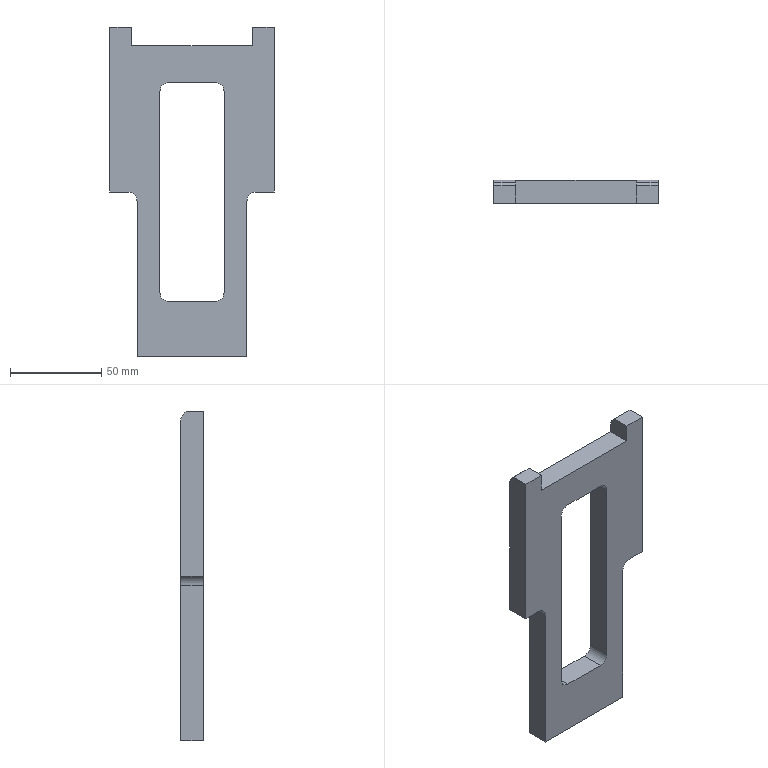Part | SolidWorks | features Fillet 3, Cut 2, Chamfer 1, Extrusion 1, ICE 1 | 1 solid | 28 faces | box 90 x 12.5 x 180 mm | volume 108281 mm3 | plane 20 | cylinder 8 | commonest cylinder face diameters 10 x8
STEP:
#1=CARTESIAN_POINT('',(45.,-6.25,180.));
#2=VERTEX_POINT('',#1);
#3=CARTESIAN_POINT('',(45.,3.25,180.));
#4=VERTEX_POINT('',#3);
#5=CARTESIAN_POINT('',(45.,6.25,180.));
#6=DIRECTION('',(0.,1.,0.));
#7=VECTOR('',#6,1000.);
#8=LINE('',#5,#7);
#9=EDGE_CURVE('',#2,#4,#8,.T.);
#10=ORIENTED_EDGE('',*,*,#9,.T.);
#11=CARTESIAN_POINT('',(33.,3.25,180.));
#12=VERTEX_POINT('',#11);
#13=CARTESIAN_POINT('',(33.,3.25,180.));
#14=DIRECTION('',(-1.,0.,0.));
#15=VECTOR('',#14,1000.);
#16=LINE('',#13,#15);
#17=EDGE_CURVE('',#4,#12,#16,.T.);
#18=ORIENTED_EDGE('',*,*,#17,.T.);
#19=CARTESIAN_POINT('',(33.,-6.25,180.));
#20=VERTEX_POINT('',#19);
#21=CARTESIAN_POINT('',(33.,-6.25,180.));
#22=DIRECTION('',(0.,1.,0.));
#23=VECTOR('',#22,1000.);
#24=LINE('',#21,#23);
#25=EDGE_CURVE('',#20,#12,#24,.T.);
#26=ORIENTED_EDGE('',*,*,#25,.F.);
#27=CARTESIAN_POINT('',(-45.,-6.25,180.));
#28=DIRECTION('',(1.,0.,0.));
#29=VECTOR('',#28,1000.);
#30=LINE('',#27,#29);
#31=EDGE_CURVE('',#20,#2,#30,.T.);
#32=ORIENTED_EDGE('',*,*,#31,.T.);
#33=EDGE_LOOP('',(#10,#18,#26,#32));
#34=FACE_OUTER_BOUND('',#33,.T.);
#35=CARTESIAN_POINT('',(0.,0.,180.));
#36=DIRECTION('',(0.,0.,1.));
#37=DIRECTION('',(1.,0.,0.));
#38=AXIS2_PLACEMENT_3D('',#35,#36,#37);
#39=PLANE('',#38);
#40=ADVANCED_FACE('',(#34),#39,.T.);
#41=CARTESIAN_POINT('',(-45.,6.25,174.929));
#42=VERTEX_POINT('',#41);
#43=CARTESIAN_POINT('',(-45.,6.25,90.));
#44=VERTEX_POINT('',#43);
#45=CARTESIAN_POINT('',(-45.,6.25,180.));
#46=DIRECTION('',(0.,0.,-1.));
#47=VECTOR('',#46,1000.);
#48=LINE('',#45,#47);
#49=EDGE_CURVE('',#42,#44,#48,.T.);
#50=ORIENTED_EDGE('',*,*,#49,.T.);
#51=CARTESIAN_POINT('',(-45.,-6.25,90.));
#52=VERTEX_POINT('',#51);
#53=CARTESIAN_POINT('',(-45.,-6.25,90.));
#54=DIRECTION('',(0.,1.,0.));
#55=VECTOR('',#54,1000.);
#56=LINE('',#53,#55);
#57=EDGE_CURVE('',#52,#44,#56,.T.);
#58=ORIENTED_EDGE('',*,*,#57,.F.);
#59=CARTESIAN_POINT('',(-45.,-6.25,180.));
#60=VERTEX_POINT('',#59);
#61=CARTESIAN_POINT('',(-45.,-6.25,180.));
#62=DIRECTION('',(0.,0.,-1.));
#63=VECTOR('',#62,1000.);
#64=LINE('',#61,#63);
#65=EDGE_CURVE('',#60,#52,#64,.T.);
#66=ORIENTED_EDGE('',*,*,#65,.F.);
#67=CARTESIAN_POINT('',(-45.,3.25,180.));
#68=VERTEX_POINT('',#67);
#69=CARTESIAN_POINT('',(-45.,6.25,180.));
#70=DIRECTION('',(0.,-1.,0.));
#71=VECTOR('',#70,1000.);
#72=LINE('',#69,#71);
#73=EDGE_CURVE('',#68,#60,#72,.T.);
#74=ORIENTED_EDGE('',*,*,#73,.F.);
#75=CARTESIAN_POINT('',(-45.,4.786,178.464));
#76=VERTEX_POINT('',#75);
#77=CARTESIAN_POINT('',(-45.,3.25,180.));
#78=DIRECTION('',(0.,0.7071,-0.7071));
#79=VECTOR('',#78,1000.);
#80=LINE('',#77,#79);
#81=EDGE_CURVE('',#68,#76,#80,.T.);
#82=ORIENTED_EDGE('',*,*,#81,.T.);
#83=CARTESIAN_POINT('',(-45.,1.25,174.929));
#84=DIRECTION('',(-1.,0.,0.));
#85=DIRECTION('',(0.,0.,-1.));
#86=AXIS2_PLACEMENT_3D('',#83,#84,#85);
#87=CIRCLE('',#86,5.);
#88=EDGE_CURVE('',#76,#42,#87,.T.);
#89=ORIENTED_EDGE('',*,*,#88,.T.);
#90=EDGE_LOOP('',(#50,#58,#66,#74,#82,#89));
#91=FACE_OUTER_BOUND('',#90,.T.);
#92=CARTESIAN_POINT('',(-45.,6.25,180.));
#93=DIRECTION('',(1.,0.,0.));
#94=DIRECTION('',(0.,0.,-1.));
#95=AXIS2_PLACEMENT_3D('',#92,#93,#94);
#96=PLANE('',#95);
#97=ADVANCED_FACE('',(#91),#96,.F.);
#98=CARTESIAN_POINT('',(17.5,-6.25,145.));
#99=VERTEX_POINT('',#98);
#100=CARTESIAN_POINT('',(17.5,-6.25,35.));
#101=VERTEX_POINT('',#100);
#102=CARTESIAN_POINT('',(17.5,-6.25,150.));
#103=DIRECTION('',(0.,0.,-1.));
#104=VECTOR('',#103,1000.);
#105=LINE('',#102,#104);
#106=EDGE_CURVE('',#99,#101,#105,.T.);
#107=ORIENTED_EDGE('',*,*,#106,.T.);
#108=CARTESIAN_POINT('',(12.5,-6.25,30.));
#109=VERTEX_POINT('',#108);
#110=CARTESIAN_POINT('',(12.5,-6.25,35.));
#111=DIRECTION('',(0.,1.,0.));
#112=DIRECTION('',(0.,0.,1.));
#113=AXIS2_PLACEMENT_3D('',#110,#111,#112);
#114=CIRCLE('',#113,5.);
#115=EDGE_CURVE('',#101,#109,#114,.T.);
#116=ORIENTED_EDGE('',*,*,#115,.T.);
#117=CARTESIAN_POINT('',(-12.5,-6.25,30.));
#118=VERTEX_POINT('',#117);
#119=CARTESIAN_POINT('',(-17.5,-6.25,30.));
#120=DIRECTION('',(-1.,0.,0.));
#121=VECTOR('',#120,1000.);
#122=LINE('',#119,#121);
#123=EDGE_CURVE('',#109,#118,#122,.T.);
#124=ORIENTED_EDGE('',*,*,#123,.T.);
#125=CARTESIAN_POINT('',(-17.5,-6.25,35.));
#126=VERTEX_POINT('',#125);
#127=CARTESIAN_POINT('',(-12.5,-6.25,35.));
#128=DIRECTION('',(0.,1.,0.));
#129=DIRECTION('',(0.,0.,1.));
#130=AXIS2_PLACEMENT_3D('',#127,#128,#129);
#131=CIRCLE('',#130,5.);
#132=EDGE_CURVE('',#118,#126,#131,.T.);
#133=ORIENTED_EDGE('',*,*,#132,.T.);
#134=CARTESIAN_POINT('',(-17.5,-6.25,145.));
#135=VERTEX_POINT('',#134);
#136=CARTESIAN_POINT('',(-17.5,-6.25,150.));
#137=DIRECTION('',(0.,0.,1.));
#138=VECTOR('',#137,1000.);
#139=LINE('',#136,#138);
#140=EDGE_CURVE('',#126,#135,#139,.T.);
#141=ORIENTED_EDGE('',*,*,#140,.T.);
#142=CARTESIAN_POINT('',(-12.5,-6.25,150.));
#143=VERTEX_POINT('',#142);
#144=CARTESIAN_POINT('',(-12.5,-6.25,145.));
#145=DIRECTION('',(0.,1.,0.));
#146=DIRECTION('',(0.,0.,1.));
#147=AXIS2_PLACEMENT_3D('',#144,#145,#146);
#148=CIRCLE('',#147,5.);
#149=EDGE_CURVE('',#135,#143,#148,.T.);
#150=ORIENTED_EDGE('',*,*,#149,.T.);
#151=CARTESIAN_POINT('',(12.5,-6.25,150.));
#152=VERTEX_POINT('',#151);
#153=CARTESIAN_POINT('',(-17.5,-6.25,150.));
#154=DIRECTION('',(1.,0.,0.));
#155=VECTOR('',#154,1000.);
#156=LINE('',#153,#155);
#157=EDGE_CURVE('',#143,#152,#156,.T.);
#158=ORIENTED_EDGE('',*,*,#157,.T.);
#159=CARTESIAN_POINT('',(12.5,-6.25,145.));
#160=DIRECTION('',(0.,1.,0.));
#161=DIRECTION('',(0.,0.,1.));
#162=AXIS2_PLACEMENT_3D('',#159,#160,#161);
#163=CIRCLE('',#162,5.);
#164=EDGE_CURVE('',#152,#99,#163,.T.);
#165=ORIENTED_EDGE('',*,*,#164,.T.);
#166=EDGE_LOOP('',(#107,#116,#124,#133,#141,#150,#158,#165));
#167=FACE_BOUND('',#166,.T.);
#168=CARTESIAN_POINT('',(-35.,-6.25,90.));
#169=VERTEX_POINT('',#168);
#170=CARTESIAN_POINT('',(-45.,-6.25,90.));
#171=DIRECTION('',(1.,0.,0.));
#172=VECTOR('',#171,1000.);
#173=LINE('',#170,#172);
#174=EDGE_CURVE('',#52,#169,#173,.T.);
#175=ORIENTED_EDGE('',*,*,#174,.T.);
#176=CARTESIAN_POINT('',(-30.,-6.25,85.));
#177=VERTEX_POINT('',#176);
#178=CARTESIAN_POINT('',(-35.,-6.25,85.));
#179=DIRECTION('',(0.,1.,0.));
#180=DIRECTION('',(0.,0.,1.));
#181=AXIS2_PLACEMENT_3D('',#178,#179,#180);
#182=CIRCLE('',#181,5.);
#183=EDGE_CURVE('',#169,#177,#182,.T.);
#184=ORIENTED_EDGE('',*,*,#183,.T.);
#185=CARTESIAN_POINT('',(-30.,-6.25,0.));
#186=VERTEX_POINT('',#185);
#187=CARTESIAN_POINT('',(-30.,-6.25,90.));
#188=DIRECTION('',(0.,0.,-1.));
#189=VECTOR('',#188,1000.);
#190=LINE('',#187,#189);
#191=EDGE_CURVE('',#177,#186,#190,.T.);
#192=ORIENTED_EDGE('',*,*,#191,.T.);
#193=CARTESIAN_POINT('',(30.,-6.25,0.));
#194=VERTEX_POINT('',#193);
#195=CARTESIAN_POINT('',(-45.,-6.25,0.));
#196=DIRECTION('',(1.,0.,0.));
#197=VECTOR('',#196,1000.);
#198=LINE('',#195,#197);
#199=EDGE_CURVE('',#186,#194,#198,.T.);
#200=ORIENTED_EDGE('',*,*,#199,.T.);
#201=CARTESIAN_POINT('',(30.,-6.25,85.));
#202=VERTEX_POINT('',#201);
#203=CARTESIAN_POINT('',(30.,-6.25,0.));
#204=DIRECTION('',(0.,0.,1.));
#205=VECTOR('',#204,1000.);
#206=LINE('',#203,#205);
#207=EDGE_CURVE('',#194,#202,#206,.T.);
#208=ORIENTED_EDGE('',*,*,#207,.T.);
#209=CARTESIAN_POINT('',(35.,-6.25,90.));
#210=VERTEX_POINT('',#209);
#211=CARTESIAN_POINT('',(35.,-6.25,85.));
#212=DIRECTION('',(0.,1.,0.));
#213=DIRECTION('',(0.,0.,1.));
#214=AXIS2_PLACEMENT_3D('',#211,#212,#213);
#215=CIRCLE('',#214,5.);
#216=EDGE_CURVE('',#202,#210,#215,.T.);
#217=ORIENTED_EDGE('',*,*,#216,.T.);
#218=CARTESIAN_POINT('',(45.,-6.25,90.));
#219=VERTEX_POINT('',#218);
#220=CARTESIAN_POINT('',(45.,-6.25,90.));
#221=DIRECTION('',(1.,0.,0.));
#222=VECTOR('',#221,1000.);
#223=LINE('',#220,#222);
#224=EDGE_CURVE('',#210,#219,#223,.T.);
#225=ORIENTED_EDGE('',*,*,#224,.T.);
#226=CARTESIAN_POINT('',(45.,-6.25,180.));
#227=DIRECTION('',(0.,0.,-1.));
#228=VECTOR('',#227,1000.);
#229=LINE('',#226,#228);
#230=EDGE_CURVE('',#2,#219,#229,.T.);
#231=ORIENTED_EDGE('',*,*,#230,.F.);
#232=ORIENTED_EDGE('',*,*,#31,.F.);
#233=CARTESIAN_POINT('',(33.,-6.25,170.));
#234=VERTEX_POINT('',#233);
#235=CARTESIAN_POINT('',(33.,-6.25,180.));
#236=DIRECTION('',(0.,0.,-1.));
#237=VECTOR('',#236,1000.);
#238=LINE('',#235,#237);
#239=EDGE_CURVE('',#20,#234,#238,.T.);
#240=ORIENTED_EDGE('',*,*,#239,.T.);
#241=CARTESIAN_POINT('',(-33.,-6.25,170.));
#242=VERTEX_POINT('',#241);
#243=CARTESIAN_POINT('',(33.,-6.25,170.));
#244=DIRECTION('',(-1.,0.,0.));
#245=VECTOR('',#244,1000.);
#246=LINE('',#243,#245);
#247=EDGE_CURVE('',#234,#242,#246,.T.);
#248=ORIENTED_EDGE('',*,*,#247,.T.);
#249=CARTESIAN_POINT('',(-33.,-6.25,180.));
#250=VERTEX_POINT('',#249);
#251=CARTESIAN_POINT('',(-33.,-6.25,180.));
#252=DIRECTION('',(0.,0.,1.));
#253=VECTOR('',#252,1000.);
#254=LINE('',#251,#253);
#255=EDGE_CURVE('',#242,#250,#254,.T.);
#256=ORIENTED_EDGE('',*,*,#255,.T.);
#257=CARTESIAN_POINT('',(-45.,-6.25,180.));
#258=DIRECTION('',(1.,0.,0.));
#259=VECTOR('',#258,1000.);
#260=LINE('',#257,#259);
#261=EDGE_CURVE('',#60,#250,#260,.T.);
#262=ORIENTED_EDGE('',*,*,#261,.F.);
#263=ORIENTED_EDGE('',*,*,#65,.T.);
#264=EDGE_LOOP('',(#175,#184,#192,#200,#208,#217,#225,#231,#232,#240,#248,#256,#262,#263));
#265=FACE_OUTER_BOUND('',#264,.T.);
#266=CARTESIAN_POINT('',(-45.,-6.25,180.));
#267=DIRECTION('',(0.,1.,0.));
#268=DIRECTION('',(0.,0.,1.));
#269=AXIS2_PLACEMENT_3D('',#266,#267,#268);
#270=PLANE('',#269);
#271=ADVANCED_FACE('',(#167,#265),#270,.F.);
#272=ORIENTED_EDGE('',*,*,#230,.T.);
#273=CARTESIAN_POINT('',(45.,6.25,90.));
#274=VERTEX_POINT('',#273);
#275=CARTESIAN_POINT('',(45.,-6.25,90.));
#276=DIRECTION('',(0.,1.,0.));
#277=VECTOR('',#276,1000.);
#278=LINE('',#275,#277);
#279=EDGE_CURVE('',#219,#274,#278,.T.);
#280=ORIENTED_EDGE('',*,*,#279,.T.);
#281=CARTESIAN_POINT('',(45.,6.25,174.929));
#282=VERTEX_POINT('',#281);
#283=CARTESIAN_POINT('',(45.,6.25,180.));
#284=DIRECTION('',(0.,0.,-1.));
#285=VECTOR('',#284,1000.);
#286=LINE('',#283,#285);
#287=EDGE_CURVE('',#282,#274,#286,.T.);
#288=ORIENTED_EDGE('',*,*,#287,.F.);
#289=CARTESIAN_POINT('',(45.,4.786,178.464));
#290=VERTEX_POINT('',#289);
#291=CARTESIAN_POINT('',(45.,1.25,174.929));
#292=DIRECTION('',(1.,0.,0.));
#293=DIRECTION('',(0.,0.,1.));
#294=AXIS2_PLACEMENT_3D('',#291,#292,#293);
#295=CIRCLE('',#294,5.);
#296=EDGE_CURVE('',#282,#290,#295,.T.);
#297=ORIENTED_EDGE('',*,*,#296,.T.);
#298=CARTESIAN_POINT('',(45.,3.25,180.));
#299=DIRECTION('',(0.,-0.7071,0.7071));
#300=VECTOR('',#299,1000.);
#301=LINE('',#298,#300);
#302=EDGE_CURVE('',#290,#4,#301,.T.);
#303=ORIENTED_EDGE('',*,*,#302,.T.);
#304=ORIENTED_EDGE('',*,*,#9,.F.);
#305=EDGE_LOOP('',(#272,#280,#288,#297,#303,#304));
#306=FACE_OUTER_BOUND('',#305,.T.);
#307=CARTESIAN_POINT('',(45.,6.25,180.));
#308=DIRECTION('',(-1.,0.,0.));
#309=DIRECTION('',(0.,0.,1.));
#310=AXIS2_PLACEMENT_3D('',#307,#308,#309);
#311=PLANE('',#310);
#312=ADVANCED_FACE('',(#306),#311,.F.);
#313=CARTESIAN_POINT('',(-12.5,6.25,150.));
#314=VERTEX_POINT('',#313);
#315=CARTESIAN_POINT('',(12.5,6.25,150.));
#316=VERTEX_POINT('',#315);
#317=CARTESIAN_POINT('',(-17.5,6.25,150.));
#318=DIRECTION('',(1.,0.,0.));
#319=VECTOR('',#318,1000.);
#320=LINE('',#317,#319);
#321=EDGE_CURVE('',#314,#316,#320,.T.);
#322=ORIENTED_EDGE('',*,*,#321,.F.);
#323=CARTESIAN_POINT('',(-17.5,6.25,145.));
#324=VERTEX_POINT('',#323);
#325=CARTESIAN_POINT('',(-12.5,6.25,145.));
#326=DIRECTION('',(0.,-1.,0.));
#327=DIRECTION('',(1.,0.,0.));
#328=AXIS2_PLACEMENT_3D('',#325,#326,#327);
#329=CIRCLE('',#328,5.);
#330=EDGE_CURVE('',#314,#324,#329,.T.);
#331=ORIENTED_EDGE('',*,*,#330,.T.);
#332=CARTESIAN_POINT('',(-17.5,6.25,35.));
#333=VERTEX_POINT('',#332);
#334=CARTESIAN_POINT('',(-17.5,6.25,150.));
#335=DIRECTION('',(0.,0.,1.));
#336=VECTOR('',#335,1000.);
#337=LINE('',#334,#336);
#338=EDGE_CURVE('',#333,#324,#337,.T.);
#339=ORIENTED_EDGE('',*,*,#338,.F.);
#340=CARTESIAN_POINT('',(-12.5,6.25,30.));
#341=VERTEX_POINT('',#340);
#342=CARTESIAN_POINT('',(-12.5,6.25,35.));
#343=DIRECTION('',(0.,-1.,0.));
#344=DIRECTION('',(1.,0.,0.));
#345=AXIS2_PLACEMENT_3D('',#342,#343,#344);
#346=CIRCLE('',#345,5.);
#347=EDGE_CURVE('',#333,#341,#346,.T.);
#348=ORIENTED_EDGE('',*,*,#347,.T.);
#349=CARTESIAN_POINT('',(12.5,6.25,30.));
#350=VERTEX_POINT('',#349);
#351=CARTESIAN_POINT('',(-17.5,6.25,30.));
#352=DIRECTION('',(-1.,0.,0.));
#353=VECTOR('',#352,1000.);
#354=LINE('',#351,#353);
#355=EDGE_CURVE('',#350,#341,#354,.T.);
#356=ORIENTED_EDGE('',*,*,#355,.F.);
#357=CARTESIAN_POINT('',(17.5,6.25,35.));
#358=VERTEX_POINT('',#357);
#359=CARTESIAN_POINT('',(12.5,6.25,35.));
#360=DIRECTION('',(0.,-1.,0.));
#361=DIRECTION('',(1.,0.,0.));
#362=AXIS2_PLACEMENT_3D('',#359,#360,#361);
#363=CIRCLE('',#362,5.);
#364=EDGE_CURVE('',#350,#358,#363,.T.);
#365=ORIENTED_EDGE('',*,*,#364,.T.);
#366=CARTESIAN_POINT('',(17.5,6.25,145.));
#367=VERTEX_POINT('',#366);
#368=CARTESIAN_POINT('',(17.5,6.25,150.));
#369=DIRECTION('',(0.,0.,-1.));
#370=VECTOR('',#369,1000.);
#371=LINE('',#368,#370);
#372=EDGE_CURVE('',#367,#358,#371,.T.);
#373=ORIENTED_EDGE('',*,*,#372,.F.);
#374=CARTESIAN_POINT('',(12.5,6.25,145.));
#375=DIRECTION('',(0.,-1.,0.));
#376=DIRECTION('',(1.,0.,0.));
#377=AXIS2_PLACEMENT_3D('',#374,#375,#376);
#378=CIRCLE('',#377,5.);
#379=EDGE_CURVE('',#367,#316,#378,.T.);
#380=ORIENTED_EDGE('',*,*,#379,.T.);
#381=EDGE_LOOP('',(#322,#331,#339,#348,#356,#365,#373,#380));
#382=FACE_BOUND('',#381,.T.);
#383=CARTESIAN_POINT('',(30.,6.25,0.));
#384=VERTEX_POINT('',#383);
#385=CARTESIAN_POINT('',(-30.,6.25,0.));
#386=VERTEX_POINT('',#385);
#387=CARTESIAN_POINT('',(-45.,6.25,0.));
#388=DIRECTION('',(-1.,0.,0.));
#389=VECTOR('',#388,1000.);
#390=LINE('',#387,#389);
#391=EDGE_CURVE('',#384,#386,#390,.T.);
#392=ORIENTED_EDGE('',*,*,#391,.T.);
#393=CARTESIAN_POINT('',(-30.,6.25,85.));
#394=VERTEX_POINT('',#393);
#395=CARTESIAN_POINT('',(-30.,6.25,90.));
#396=DIRECTION('',(0.,0.,-1.));
#397=VECTOR('',#396,1000.);
#398=LINE('',#395,#397);
#399=EDGE_CURVE('',#394,#386,#398,.T.);
#400=ORIENTED_EDGE('',*,*,#399,.F.);
#401=CARTESIAN_POINT('',(-35.,6.25,90.));
#402=VERTEX_POINT('',#401);
#403=CARTESIAN_POINT('',(-35.,6.25,85.));
#404=DIRECTION('',(0.,-1.,0.));
#405=DIRECTION('',(1.,0.,0.));
#406=AXIS2_PLACEMENT_3D('',#403,#404,#405);
#407=CIRCLE('',#406,5.);
#408=EDGE_CURVE('',#394,#402,#407,.T.);
#409=ORIENTED_EDGE('',*,*,#408,.T.);
#410=CARTESIAN_POINT('',(-45.,6.25,90.));
#411=DIRECTION('',(1.,0.,0.));
#412=VECTOR('',#411,1000.);
#413=LINE('',#410,#412);
#414=EDGE_CURVE('',#44,#402,#413,.T.);
#415=ORIENTED_EDGE('',*,*,#414,.F.);
#416=ORIENTED_EDGE('',*,*,#49,.F.);
#417=CARTESIAN_POINT('',(-33.,6.25,174.929));
#418=VERTEX_POINT('',#417);
#419=CARTESIAN_POINT('',(-33.,6.25,174.929));
#420=DIRECTION('',(1.,0.,0.));
#421=VECTOR('',#420,1000.);
#422=LINE('',#419,#421);
#423=EDGE_CURVE('',#42,#418,#422,.T.);
#424=ORIENTED_EDGE('',*,*,#423,.T.);
#425=CARTESIAN_POINT('',(-33.,6.25,170.));
#426=VERTEX_POINT('',#425);
#427=CARTESIAN_POINT('',(-33.,6.25,180.));
#428=DIRECTION('',(0.,0.,1.));
#429=VECTOR('',#428,1000.);
#430=LINE('',#427,#429);
#431=EDGE_CURVE('',#426,#418,#430,.T.);
#432=ORIENTED_EDGE('',*,*,#431,.F.);
#433=CARTESIAN_POINT('',(33.,6.25,170.));
#434=VERTEX_POINT('',#433);
#435=CARTESIAN_POINT('',(33.,6.25,170.));
#436=DIRECTION('',(-1.,0.,0.));
#437=VECTOR('',#436,1000.);
#438=LINE('',#435,#437);
#439=EDGE_CURVE('',#434,#426,#438,.T.);
#440=ORIENTED_EDGE('',*,*,#439,.F.);
#441=CARTESIAN_POINT('',(33.,6.25,174.929));
#442=VERTEX_POINT('',#441);
#443=CARTESIAN_POINT('',(33.,6.25,180.));
#444=DIRECTION('',(0.,0.,-1.));
#445=VECTOR('',#444,1000.);
#446=LINE('',#443,#445);
#447=EDGE_CURVE('',#442,#434,#446,.T.);
#448=ORIENTED_EDGE('',*,*,#447,.F.);
#449=CARTESIAN_POINT('',(45.,6.25,174.929));
#450=DIRECTION('',(1.,0.,0.));
#451=VECTOR('',#450,1000.);
#452=LINE('',#449,#451);
#453=EDGE_CURVE('',#442,#282,#452,.T.);
#454=ORIENTED_EDGE('',*,*,#453,.T.);
#455=ORIENTED_EDGE('',*,*,#287,.T.);
#456=CARTESIAN_POINT('',(35.,6.25,90.));
#457=VERTEX_POINT('',#456);
#458=CARTESIAN_POINT('',(45.,6.25,90.));
#459=DIRECTION('',(1.,0.,0.));
#460=VECTOR('',#459,1000.);
#461=LINE('',#458,#460);
#462=EDGE_CURVE('',#457,#274,#461,.T.);
#463=ORIENTED_EDGE('',*,*,#462,.F.);
#464=CARTESIAN_POINT('',(30.,6.25,85.));
#465=VERTEX_POINT('',#464);
#466=CARTESIAN_POINT('',(35.,6.25,85.));
#467=DIRECTION('',(0.,-1.,0.));
#468=DIRECTION('',(1.,0.,0.));
#469=AXIS2_PLACEMENT_3D('',#466,#467,#468);
#470=CIRCLE('',#469,5.);
#471=EDGE_CURVE('',#457,#465,#470,.T.);
#472=ORIENTED_EDGE('',*,*,#471,.T.);
#473=CARTESIAN_POINT('',(30.,6.25,0.));
#474=DIRECTION('',(0.,0.,1.));
#475=VECTOR('',#474,1000.);
#476=LINE('',#473,#475);
#477=EDGE_CURVE('',#384,#465,#476,.T.);
#478=ORIENTED_EDGE('',*,*,#477,.F.);
#479=EDGE_LOOP('',(#392,#400,#409,#415,#416,#424,#432,#440,#448,#454,#455,#463,#472,#478));
#480=FACE_OUTER_BOUND('',#479,.T.);
#481=CARTESIAN_POINT('',(-45.,6.25,180.));
#482=DIRECTION('',(0.,-1.,0.));
#483=DIRECTION('',(1.,0.,0.));
#484=AXIS2_PLACEMENT_3D('',#481,#482,#483);
#485=PLANE('',#484);
#486=ADVANCED_FACE('',(#382,#480),#485,.F.);
#487=CARTESIAN_POINT('',(-33.,3.25,180.));
#488=VERTEX_POINT('',#487);
#489=CARTESIAN_POINT('',(-33.,-6.25,180.));
#490=DIRECTION('',(0.,1.,0.));
#491=VECTOR('',#490,1000.);
#492=LINE('',#489,#491);
#493=EDGE_CURVE('',#250,#488,#492,.T.);
#494=ORIENTED_EDGE('',*,*,#493,.T.);
#495=CARTESIAN_POINT('',(-45.,3.25,180.));
#496=DIRECTION('',(-1.,0.,0.));
#497=VECTOR('',#496,1000.);
#498=LINE('',#495,#497);
#499=EDGE_CURVE('',#488,#68,#498,.T.);
#500=ORIENTED_EDGE('',*,*,#499,.T.);
#501=ORIENTED_EDGE('',*,*,#73,.T.);
#502=ORIENTED_EDGE('',*,*,#261,.T.);
#503=EDGE_LOOP('',(#494,#500,#501,#502));
#504=FACE_OUTER_BOUND('',#503,.T.);
#505=CARTESIAN_POINT('',(0.,0.,180.));
#506=DIRECTION('',(0.,0.,1.));
#507=DIRECTION('',(1.,0.,0.));
#508=AXIS2_PLACEMENT_3D('',#505,#506,#507);
#509=PLANE('',#508);
#510=ADVANCED_FACE('',(#504),#509,.T.);
#511=ORIENTED_EDGE('',*,*,#199,.F.);
#512=CARTESIAN_POINT('',(-30.,-6.25,0.));
#513=DIRECTION('',(0.,1.,0.));
#514=VECTOR('',#513,1000.);
#515=LINE('',#512,#514);
#516=EDGE_CURVE('',#186,#386,#515,.T.);
#517=ORIENTED_EDGE('',*,*,#516,.T.);
#518=ORIENTED_EDGE('',*,*,#391,.F.);
#519=CARTESIAN_POINT('',(30.,-6.25,0.));
#520=DIRECTION('',(0.,1.,0.));
#521=VECTOR('',#520,1000.);
#522=LINE('',#519,#521);
#523=EDGE_CURVE('',#194,#384,#522,.T.);
#524=ORIENTED_EDGE('',*,*,#523,.F.);
#525=EDGE_LOOP('',(#511,#517,#518,#524));
#526=FACE_OUTER_BOUND('',#525,.T.);
#527=CARTESIAN_POINT('',(0.,0.,0.));
#528=DIRECTION('',(0.,0.,1.));
#529=DIRECTION('',(1.,0.,0.));
#530=AXIS2_PLACEMENT_3D('',#527,#528,#529);
#531=PLANE('',#530);
#532=ADVANCED_FACE('',(#526),#531,.F.);
#533=CARTESIAN_POINT('',(33.,4.786,178.464));
#534=VERTEX_POINT('',#533);
#535=CARTESIAN_POINT('',(33.,3.25,180.));
#536=DIRECTION('',(0.,0.7071,-0.7071));
#537=VECTOR('',#536,1000.);
#538=LINE('',#535,#537);
#539=EDGE_CURVE('',#12,#534,#538,.T.);
#540=ORIENTED_EDGE('',*,*,#539,.T.);
#541=CARTESIAN_POINT('',(33.,1.25,174.929));
#542=DIRECTION('',(-1.,0.,0.));
#543=DIRECTION('',(0.,1.,0.));
#544=AXIS2_PLACEMENT_3D('',#541,#542,#543);
#545=CIRCLE('',#544,5.);
#546=EDGE_CURVE('',#534,#442,#545,.T.);
#547=ORIENTED_EDGE('',*,*,#546,.T.);
#548=ORIENTED_EDGE('',*,*,#447,.T.);
#549=CARTESIAN_POINT('',(33.,-6.25,170.));
#550=DIRECTION('',(0.,1.,0.));
#551=VECTOR('',#550,1000.);
#552=LINE('',#549,#551);
#553=EDGE_CURVE('',#234,#434,#552,.T.);
#554=ORIENTED_EDGE('',*,*,#553,.F.);
#555=ORIENTED_EDGE('',*,*,#239,.F.);
#556=ORIENTED_EDGE('',*,*,#25,.T.);
#557=EDGE_LOOP('',(#540,#547,#548,#554,#555,#556));
#558=FACE_OUTER_BOUND('',#557,.T.);
#559=CARTESIAN_POINT('',(33.,-6.25,180.));
#560=DIRECTION('',(1.,0.,0.));
#561=DIRECTION('',(0.,1.,0.));
#562=AXIS2_PLACEMENT_3D('',#559,#560,#561);
#563=PLANE('',#562);
#564=ADVANCED_FACE('',(#558),#563,.F.);
#565=ORIENTED_EDGE('',*,*,#431,.T.);
#566=CARTESIAN_POINT('',(-33.,4.786,178.464));
#567=VERTEX_POINT('',#566);
#568=CARTESIAN_POINT('',(-33.,1.25,174.929));
#569=DIRECTION('',(1.,0.,0.));
#570=DIRECTION('',(0.,-1.,0.));
#571=AXIS2_PLACEMENT_3D('',#568,#569,#570);
#572=CIRCLE('',#571,5.);
#573=EDGE_CURVE('',#418,#567,#572,.T.);
#574=ORIENTED_EDGE('',*,*,#573,.T.);
#575=CARTESIAN_POINT('',(-33.,3.25,180.));
#576=DIRECTION('',(0.,-0.7071,0.7071));
#577=VECTOR('',#576,1000.);
#578=LINE('',#575,#577);
#579=EDGE_CURVE('',#567,#488,#578,.T.);
#580=ORIENTED_EDGE('',*,*,#579,.T.);
#581=ORIENTED_EDGE('',*,*,#493,.F.);
#582=ORIENTED_EDGE('',*,*,#255,.F.);
#583=CARTESIAN_POINT('',(-33.,-6.25,170.));
#584=DIRECTION('',(0.,1.,0.));
#585=VECTOR('',#584,1000.);
#586=LINE('',#583,#585);
#587=EDGE_CURVE('',#242,#426,#586,.T.);
#588=ORIENTED_EDGE('',*,*,#587,.T.);
#589=EDGE_LOOP('',(#565,#574,#580,#581,#582,#588));
#590=FACE_OUTER_BOUND('',#589,.T.);
#591=CARTESIAN_POINT('',(-33.,-6.25,180.));
#592=DIRECTION('',(-1.,0.,0.));
#593=DIRECTION('',(0.,-1.,0.));
#594=AXIS2_PLACEMENT_3D('',#591,#592,#593);
#595=PLANE('',#594);
#596=ADVANCED_FACE('',(#590),#595,.F.);
#597=ORIENTED_EDGE('',*,*,#439,.T.);
#598=ORIENTED_EDGE('',*,*,#587,.F.);
#599=ORIENTED_EDGE('',*,*,#247,.F.);
#600=ORIENTED_EDGE('',*,*,#553,.T.);
#601=EDGE_LOOP('',(#597,#598,#599,#600));
#602=FACE_OUTER_BOUND('',#601,.T.);
#603=CARTESIAN_POINT('',(33.,-6.25,170.));
#604=DIRECTION('',(0.,0.,-1.));
#605=DIRECTION('',(-1.,0.,0.));
#606=AXIS2_PLACEMENT_3D('',#603,#604,#605);
#607=PLANE('',#606);
#608=ADVANCED_FACE('',(#602),#607,.F.);
#609=ORIENTED_EDGE('',*,*,#579,.F.);
#610=CARTESIAN_POINT('',(-45.,4.786,178.464));
#611=DIRECTION('',(-1.,0.,0.));
#612=VECTOR('',#611,1000.);
#613=LINE('',#610,#612);
#614=EDGE_CURVE('',#567,#76,#613,.T.);
#615=ORIENTED_EDGE('',*,*,#614,.T.);
#616=ORIENTED_EDGE('',*,*,#81,.F.);
#617=ORIENTED_EDGE('',*,*,#499,.F.);
#618=EDGE_LOOP('',(#609,#615,#616,#617));
#619=FACE_OUTER_BOUND('',#618,.T.);
#620=CARTESIAN_POINT('',(0.,3.25,180.));
#621=DIRECTION('',(0.,0.7071,0.7071));
#622=DIRECTION('',(1.,0.,0.));
#623=AXIS2_PLACEMENT_3D('',#620,#621,#622);
#624=PLANE('',#623);
#625=ADVANCED_FACE('',(#619),#624,.T.);
#626=ORIENTED_EDGE('',*,*,#302,.F.);
#627=CARTESIAN_POINT('',(33.,4.786,178.464));
#628=DIRECTION('',(-1.,0.,0.));
#629=VECTOR('',#628,1000.);
#630=LINE('',#627,#629);
#631=EDGE_CURVE('',#290,#534,#630,.T.);
#632=ORIENTED_EDGE('',*,*,#631,.T.);
#633=ORIENTED_EDGE('',*,*,#539,.F.);
#634=ORIENTED_EDGE('',*,*,#17,.F.);
#635=EDGE_LOOP('',(#626,#632,#633,#634));
#636=FACE_OUTER_BOUND('',#635,.T.);
#637=CARTESIAN_POINT('',(0.,3.25,180.));
#638=DIRECTION('',(0.,0.7071,0.7071));
#639=DIRECTION('',(1.,0.,0.));
#640=AXIS2_PLACEMENT_3D('',#637,#638,#639);
#641=PLANE('',#640);
#642=ADVANCED_FACE('',(#636),#641,.T.);
#643=ORIENTED_EDGE('',*,*,#88,.F.);
#644=ORIENTED_EDGE('',*,*,#614,.F.);
#645=ORIENTED_EDGE('',*,*,#573,.F.);
#646=ORIENTED_EDGE('',*,*,#423,.F.);
#647=EDGE_LOOP('',(#643,#644,#645,#646));
#648=FACE_OUTER_BOUND('',#647,.T.);
#649=CARTESIAN_POINT('',(-45.,1.25,174.929));
#650=DIRECTION('',(-1.,0.,0.));
#651=DIRECTION('',(0.,-1.,0.));
#652=AXIS2_PLACEMENT_3D('',#649,#650,#651);
#653=CYLINDRICAL_SURFACE('',#652,5.);
#654=ADVANCED_FACE('',(#648),#653,.T.);
#655=ORIENTED_EDGE('',*,*,#546,.F.);
#656=ORIENTED_EDGE('',*,*,#631,.F.);
#657=ORIENTED_EDGE('',*,*,#296,.F.);
#658=ORIENTED_EDGE('',*,*,#453,.F.);
#659=EDGE_LOOP('',(#655,#656,#657,#658));
#660=FACE_OUTER_BOUND('',#659,.T.);
#661=CARTESIAN_POINT('',(-45.,1.25,174.929));
#662=DIRECTION('',(-1.,0.,0.));
#663=DIRECTION('',(0.,-1.,0.));
#664=AXIS2_PLACEMENT_3D('',#661,#662,#663);
#665=CYLINDRICAL_SURFACE('',#664,5.);
#666=ADVANCED_FACE('',(#660),#665,.T.);
#667=ORIENTED_EDGE('',*,*,#224,.F.);
#668=CARTESIAN_POINT('',(35.,6.25,90.));
#669=DIRECTION('',(0.,1.,0.));
#670=VECTOR('',#669,1000.);
#671=LINE('',#668,#670);
#672=EDGE_CURVE('',#210,#457,#671,.T.);
#673=ORIENTED_EDGE('',*,*,#672,.T.);
#674=ORIENTED_EDGE('',*,*,#462,.T.);
#675=ORIENTED_EDGE('',*,*,#279,.F.);
#676=EDGE_LOOP('',(#667,#673,#674,#675));
#677=FACE_OUTER_BOUND('',#676,.T.);
#678=CARTESIAN_POINT('',(45.,-6.25,90.));
#679=DIRECTION('',(0.,0.,1.));
#680=DIRECTION('',(1.,0.,0.));
#681=AXIS2_PLACEMENT_3D('',#678,#679,#680);
#682=PLANE('',#681);
#683=ADVANCED_FACE('',(#677),#682,.F.);
#684=ORIENTED_EDGE('',*,*,#477,.T.);
#685=CARTESIAN_POINT('',(30.,-6.25,85.));
#686=DIRECTION('',(0.,-1.,0.));
#687=VECTOR('',#686,1000.);
#688=LINE('',#685,#687);
#689=EDGE_CURVE('',#465,#202,#688,.T.);
#690=ORIENTED_EDGE('',*,*,#689,.T.);
#691=ORIENTED_EDGE('',*,*,#207,.F.);
#692=ORIENTED_EDGE('',*,*,#523,.T.);
#693=EDGE_LOOP('',(#684,#690,#691,#692));
#694=FACE_OUTER_BOUND('',#693,.T.);
#695=CARTESIAN_POINT('',(30.,-6.25,0.));
#696=DIRECTION('',(-1.,0.,0.));
#697=DIRECTION('',(0.,-1.,0.));
#698=AXIS2_PLACEMENT_3D('',#695,#696,#697);
#699=PLANE('',#698);
#700=ADVANCED_FACE('',(#694),#699,.F.);
#701=ORIENTED_EDGE('',*,*,#191,.F.);
#702=CARTESIAN_POINT('',(-30.,6.25,85.));
#703=DIRECTION('',(0.,1.,0.));
#704=VECTOR('',#703,1000.);
#705=LINE('',#702,#704);
#706=EDGE_CURVE('',#177,#394,#705,.T.);
#707=ORIENTED_EDGE('',*,*,#706,.T.);
#708=ORIENTED_EDGE('',*,*,#399,.T.);
#709=ORIENTED_EDGE('',*,*,#516,.F.);
#710=EDGE_LOOP('',(#701,#707,#708,#709));
#711=FACE_OUTER_BOUND('',#710,.T.);
#712=CARTESIAN_POINT('',(-30.,-6.25,90.));
#713=DIRECTION('',(1.,0.,0.));
#714=DIRECTION('',(0.,1.,0.));
#715=AXIS2_PLACEMENT_3D('',#712,#713,#714);
#716=PLANE('',#715);
#717=ADVANCED_FACE('',(#711),#716,.F.);
#718=ORIENTED_EDGE('',*,*,#414,.T.);
#719=CARTESIAN_POINT('',(-35.,-6.25,90.));
#720=DIRECTION('',(0.,-1.,0.));
#721=VECTOR('',#720,1000.);
#722=LINE('',#719,#721);
#723=EDGE_CURVE('',#402,#169,#722,.T.);
#724=ORIENTED_EDGE('',*,*,#723,.T.);
#725=ORIENTED_EDGE('',*,*,#174,.F.);
#726=ORIENTED_EDGE('',*,*,#57,.T.);
#727=EDGE_LOOP('',(#718,#724,#725,#726));
#728=FACE_OUTER_BOUND('',#727,.T.);
#729=CARTESIAN_POINT('',(-45.,-6.25,90.));
#730=DIRECTION('',(0.,0.,1.));
#731=DIRECTION('',(1.,0.,0.));
#732=AXIS2_PLACEMENT_3D('',#729,#730,#731);
#733=PLANE('',#732);
#734=ADVANCED_FACE('',(#728),#733,.F.);
#735=ORIENTED_EDGE('',*,*,#140,.F.);
#736=CARTESIAN_POINT('',(-17.5,6.25,35.));
#737=DIRECTION('',(0.,1.,0.));
#738=VECTOR('',#737,1000.);
#739=LINE('',#736,#738);
#740=EDGE_CURVE('',#126,#333,#739,.T.);
#741=ORIENTED_EDGE('',*,*,#740,.T.);
#742=ORIENTED_EDGE('',*,*,#338,.T.);
#743=CARTESIAN_POINT('',(-17.5,-6.25,145.));
#744=DIRECTION('',(0.,-1.,0.));
#745=VECTOR('',#744,1000.);
#746=LINE('',#743,#745);
#747=EDGE_CURVE('',#324,#135,#746,.T.);
#748=ORIENTED_EDGE('',*,*,#747,.T.);
#749=EDGE_LOOP('',(#735,#741,#742,#748));
#750=FACE_OUTER_BOUND('',#749,.T.);
#751=CARTESIAN_POINT('',(-17.5,-6.25,150.));
#752=DIRECTION('',(-1.,0.,0.));
#753=DIRECTION('',(0.,-1.,0.));
#754=AXIS2_PLACEMENT_3D('',#751,#752,#753);
#755=PLANE('',#754);
#756=ADVANCED_FACE('',(#750),#755,.F.);
#757=ORIENTED_EDGE('',*,*,#123,.F.);
#758=CARTESIAN_POINT('',(12.5,6.25,30.));
#759=DIRECTION('',(0.,1.,0.));
#760=VECTOR('',#759,1000.);
#761=LINE('',#758,#760);
#762=EDGE_CURVE('',#109,#350,#761,.T.);
#763=ORIENTED_EDGE('',*,*,#762,.T.);
#764=ORIENTED_EDGE('',*,*,#355,.T.);
#765=CARTESIAN_POINT('',(-12.5,-6.25,30.));
#766=DIRECTION('',(0.,-1.,0.));
#767=VECTOR('',#766,1000.);
#768=LINE('',#765,#767);
#769=EDGE_CURVE('',#341,#118,#768,.T.);
#770=ORIENTED_EDGE('',*,*,#769,.T.);
#771=EDGE_LOOP('',(#757,#763,#764,#770));
#772=FACE_OUTER_BOUND('',#771,.T.);
#773=CARTESIAN_POINT('',(-17.5,-6.25,30.));
#774=DIRECTION('',(0.,0.,-1.));
#775=DIRECTION('',(-1.,0.,0.));
#776=AXIS2_PLACEMENT_3D('',#773,#774,#775);
#777=PLANE('',#776);
#778=ADVANCED_FACE('',(#772),#777,.F.);
#779=ORIENTED_EDGE('',*,*,#372,.T.);
#780=CARTESIAN_POINT('',(17.5,-6.25,35.));
#781=DIRECTION('',(0.,-1.,0.));
#782=VECTOR('',#781,1000.);
#783=LINE('',#780,#782);
#784=EDGE_CURVE('',#358,#101,#783,.T.);
#785=ORIENTED_EDGE('',*,*,#784,.T.);
#786=ORIENTED_EDGE('',*,*,#106,.F.);
#787=CARTESIAN_POINT('',(17.5,6.25,145.));
#788=DIRECTION('',(0.,1.,0.));
#789=VECTOR('',#788,1000.);
#790=LINE('',#787,#789);
#791=EDGE_CURVE('',#99,#367,#790,.T.);
#792=ORIENTED_EDGE('',*,*,#791,.T.);
#793=EDGE_LOOP('',(#779,#785,#786,#792));
#794=FACE_OUTER_BOUND('',#793,.T.);
#795=CARTESIAN_POINT('',(17.5,-6.25,150.));
#796=DIRECTION('',(1.,0.,0.));
#797=DIRECTION('',(0.,1.,0.));
#798=AXIS2_PLACEMENT_3D('',#795,#796,#797);
#799=PLANE('',#798);
#800=ADVANCED_FACE('',(#794),#799,.F.);
#801=ORIENTED_EDGE('',*,*,#321,.T.);
#802=CARTESIAN_POINT('',(12.5,-6.25,150.));
#803=DIRECTION('',(0.,-1.,0.));
#804=VECTOR('',#803,1000.);
#805=LINE('',#802,#804);
#806=EDGE_CURVE('',#316,#152,#805,.T.);
#807=ORIENTED_EDGE('',*,*,#806,.T.);
#808=ORIENTED_EDGE('',*,*,#157,.F.);
#809=CARTESIAN_POINT('',(-12.5,6.25,150.));
#810=DIRECTION('',(0.,1.,0.));
#811=VECTOR('',#810,1000.);
#812=LINE('',#809,#811);
#813=EDGE_CURVE('',#143,#314,#812,.T.);
#814=ORIENTED_EDGE('',*,*,#813,.T.);
#815=EDGE_LOOP('',(#801,#807,#808,#814));
#816=FACE_OUTER_BOUND('',#815,.T.);
#817=CARTESIAN_POINT('',(-17.5,-6.25,150.));
#818=DIRECTION('',(0.,0.,1.));
#819=DIRECTION('',(1.,0.,0.));
#820=AXIS2_PLACEMENT_3D('',#817,#818,#819);
#821=PLANE('',#820);
#822=ADVANCED_FACE('',(#816),#821,.F.);
#823=ORIENTED_EDGE('',*,*,#115,.F.);
#824=ORIENTED_EDGE('',*,*,#784,.F.);
#825=ORIENTED_EDGE('',*,*,#364,.F.);
#826=ORIENTED_EDGE('',*,*,#762,.F.);
#827=EDGE_LOOP('',(#823,#824,#825,#826));
#828=FACE_OUTER_BOUND('',#827,.T.);
#829=CARTESIAN_POINT('',(12.5,-6.25,35.));
#830=DIRECTION('',(0.,-1.,0.));
#831=DIRECTION('',(1.,0.,0.));
#832=AXIS2_PLACEMENT_3D('',#829,#830,#831);
#833=CYLINDRICAL_SURFACE('',#832,5.);
#834=ADVANCED_FACE('',(#828),#833,.F.);
#835=ORIENTED_EDGE('',*,*,#132,.F.);
#836=ORIENTED_EDGE('',*,*,#769,.F.);
#837=ORIENTED_EDGE('',*,*,#347,.F.);
#838=ORIENTED_EDGE('',*,*,#740,.F.);
#839=EDGE_LOOP('',(#835,#836,#837,#838));
#840=FACE_OUTER_BOUND('',#839,.T.);
#841=CARTESIAN_POINT('',(-12.5,-6.25,35.));
#842=DIRECTION('',(0.,-1.,0.));
#843=DIRECTION('',(1.,0.,0.));
#844=AXIS2_PLACEMENT_3D('',#841,#842,#843);
#845=CYLINDRICAL_SURFACE('',#844,5.);
#846=ADVANCED_FACE('',(#840),#845,.F.);
#847=ORIENTED_EDGE('',*,*,#164,.F.);
#848=ORIENTED_EDGE('',*,*,#806,.F.);
#849=ORIENTED_EDGE('',*,*,#379,.F.);
#850=ORIENTED_EDGE('',*,*,#791,.F.);
#851=EDGE_LOOP('',(#847,#848,#849,#850));
#852=FACE_OUTER_BOUND('',#851,.T.);
#853=CARTESIAN_POINT('',(12.5,-6.25,145.));
#854=DIRECTION('',(0.,-1.,0.));
#855=DIRECTION('',(1.,0.,0.));
#856=AXIS2_PLACEMENT_3D('',#853,#854,#855);
#857=CYLINDRICAL_SURFACE('',#856,5.);
#858=ADVANCED_FACE('',(#852),#857,.F.);
#859=ORIENTED_EDGE('',*,*,#149,.F.);
#860=ORIENTED_EDGE('',*,*,#747,.F.);
#861=ORIENTED_EDGE('',*,*,#330,.F.);
#862=ORIENTED_EDGE('',*,*,#813,.F.);
#863=EDGE_LOOP('',(#859,#860,#861,#862));
#864=FACE_OUTER_BOUND('',#863,.T.);
#865=CARTESIAN_POINT('',(-12.5,-6.25,145.));
#866=DIRECTION('',(0.,-1.,0.));
#867=DIRECTION('',(1.,0.,0.));
#868=AXIS2_PLACEMENT_3D('',#865,#866,#867);
#869=CYLINDRICAL_SURFACE('',#868,5.);
#870=ADVANCED_FACE('',(#864),#869,.F.);
#871=ORIENTED_EDGE('',*,*,#183,.F.);
#872=ORIENTED_EDGE('',*,*,#723,.F.);
#873=ORIENTED_EDGE('',*,*,#408,.F.);
#874=ORIENTED_EDGE('',*,*,#706,.F.);
#875=EDGE_LOOP('',(#871,#872,#873,#874));
#876=FACE_OUTER_BOUND('',#875,.T.);
#877=CARTESIAN_POINT('',(-35.,-6.25,85.));
#878=DIRECTION('',(0.,-1.,0.));
#879=DIRECTION('',(1.,0.,0.));
#880=AXIS2_PLACEMENT_3D('',#877,#878,#879);
#881=CYLINDRICAL_SURFACE('',#880,5.);
#882=ADVANCED_FACE('',(#876),#881,.F.);
#883=ORIENTED_EDGE('',*,*,#216,.F.);
#884=ORIENTED_EDGE('',*,*,#689,.F.);
#885=ORIENTED_EDGE('',*,*,#471,.F.);
#886=ORIENTED_EDGE('',*,*,#672,.F.);
#887=EDGE_LOOP('',(#883,#884,#885,#886));
#888=FACE_OUTER_BOUND('',#887,.T.);
#889=CARTESIAN_POINT('',(35.,-6.25,85.));
#890=DIRECTION('',(0.,-1.,0.));
#891=DIRECTION('',(1.,0.,0.));
#892=AXIS2_PLACEMENT_3D('',#889,#890,#891);
#893=CYLINDRICAL_SURFACE('',#892,5.);
#894=ADVANCED_FACE('',(#888),#893,.F.);
#895=CLOSED_SHELL('',(#40,#97,#271,#312,#486,#510,#532,#564,#596,#608,#625,#642,#654,#666,#683,#700,#717,#734,#756,#778,#800,#822,#834,#846,#858,#870,#882,#894));
#896=MANIFOLD_SOLID_BREP('',#895);
#897=CARTESIAN_POINT('',(0.,0.,0.));
#898=DIRECTION('',(0.,0.,1.));
#899=DIRECTION('',(1.,0.,0.));
#900=AXIS2_PLACEMENT_3D('',#897,#898,#899);
#901=(LENGTH_UNIT()NAMED_UNIT(*)SI_UNIT(.MILLI.,.METRE.));
#902=UNCERTAINTY_MEASURE_WITH_UNIT(LENGTH_MEASURE(0.00001),#901,'','');
#903=(NAMED_UNIT(*)PLANE_ANGLE_UNIT()SI_UNIT($,.RADIAN.));
#904=(NAMED_UNIT(*)SI_UNIT($,.STERADIAN.)SOLID_ANGLE_UNIT());
#905=(GEOMETRIC_REPRESENTATION_CONTEXT(3)GLOBAL_UNCERTAINTY_ASSIGNED_CONTEXT((#902))GLOBAL_UNIT_ASSIGNED_CONTEXT((#901,#903,#904))REPRESENTATION_CONTEXT('',''));
#906=ADVANCED_BREP_SHAPE_REPRESENTATION('',(#896,#900),#905);